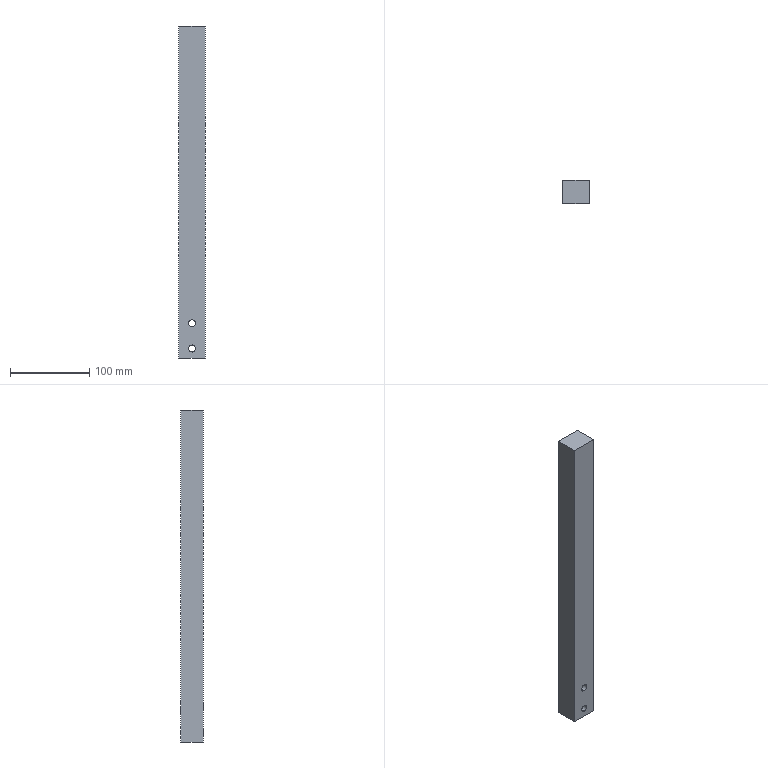Part | STEP file | zq Auxiliary Guide Rail | 1 solid | 16 faces | box 34 x 29 x 420 mm | volume 407406 mm3 | cylinder 8 | plane 8 | commonest cylinder face diameters 9 x4 16 x4
STEP:
#1=CARTESIAN_POINT('',(-17.747,48.45,16.5));
#2=VERTEX_POINT('',#1);
#3=CARTESIAN_POINT('',(-17.747,48.45,7.5));
#4=VERTEX_POINT('',#3);
#5=CARTESIAN_POINT('',(-17.747,48.45,12.));
#6=DIRECTION('',(0.,-1.,0.));
#7=DIRECTION('',(0.,0.,1.));
#8=AXIS2_PLACEMENT_3D('',#5,#6,#7);
#9=CIRCLE('',#8,4.5);
#10=EDGE_CURVE('',#2,#4,#9,.T.);
#11=ORIENTED_EDGE('',*,*,#10,.T.);
#12=CARTESIAN_POINT('',(-17.747,66.45,7.5));
#13=VERTEX_POINT('',#12);
#14=CARTESIAN_POINT('',(-17.747,47.45,7.5));
#15=DIRECTION('',(0.,1.,0.));
#16=VECTOR('',#15,1000.);
#17=LINE('',#14,#16);
#18=EDGE_CURVE('',#4,#13,#17,.T.);
#19=ORIENTED_EDGE('',*,*,#18,.T.);
#20=CARTESIAN_POINT('',(-17.747,66.45,16.5));
#21=VERTEX_POINT('',#20);
#22=CARTESIAN_POINT('',(-17.747,66.45,12.));
#23=DIRECTION('',(0.,-1.,0.));
#24=DIRECTION('',(0.,0.,1.));
#25=AXIS2_PLACEMENT_3D('',#22,#23,#24);
#26=CIRCLE('',#25,4.5);
#27=EDGE_CURVE('',#21,#13,#26,.T.);
#28=ORIENTED_EDGE('',*,*,#27,.F.);
#29=CARTESIAN_POINT('',(-17.747,47.45,16.5));
#30=DIRECTION('',(0.,1.,0.));
#31=VECTOR('',#30,1000.);
#32=LINE('',#29,#31);
#33=EDGE_CURVE('',#2,#21,#32,.T.);
#34=ORIENTED_EDGE('',*,*,#33,.F.);
#35=EDGE_LOOP('',(#11,#19,#28,#34));
#36=FACE_OUTER_BOUND('',#35,.T.);
#37=CARTESIAN_POINT('',(-17.747,47.45,12.));
#38=DIRECTION('',(0.,1.,0.));
#39=DIRECTION('',(0.,0.,1.));
#40=AXIS2_PLACEMENT_3D('',#37,#38,#39);
#41=CYLINDRICAL_SURFACE('',#40,4.5);
#42=ADVANCED_FACE('',(#36),#41,.F.);
#43=CARTESIAN_POINT('',(-17.747,48.45,48.5));
#44=VERTEX_POINT('',#43);
#45=CARTESIAN_POINT('',(-17.747,48.45,39.5));
#46=VERTEX_POINT('',#45);
#47=CARTESIAN_POINT('',(-17.747,48.45,44.));
#48=DIRECTION('',(0.,-1.,0.));
#49=DIRECTION('',(0.,0.,1.));
#50=AXIS2_PLACEMENT_3D('',#47,#48,#49);
#51=CIRCLE('',#50,4.5);
#52=EDGE_CURVE('',#44,#46,#51,.T.);
#53=ORIENTED_EDGE('',*,*,#52,.T.);
#54=CARTESIAN_POINT('',(-17.747,66.45,39.5));
#55=VERTEX_POINT('',#54);
#56=CARTESIAN_POINT('',(-17.747,47.45,39.5));
#57=DIRECTION('',(0.,1.,0.));
#58=VECTOR('',#57,1000.);
#59=LINE('',#56,#58);
#60=EDGE_CURVE('',#46,#55,#59,.T.);
#61=ORIENTED_EDGE('',*,*,#60,.T.);
#62=CARTESIAN_POINT('',(-17.747,66.45,48.5));
#63=VERTEX_POINT('',#62);
#64=CARTESIAN_POINT('',(-17.747,66.45,44.));
#65=DIRECTION('',(0.,-1.,0.));
#66=DIRECTION('',(0.,0.,1.));
#67=AXIS2_PLACEMENT_3D('',#64,#65,#66);
#68=CIRCLE('',#67,4.5);
#69=EDGE_CURVE('',#63,#55,#68,.T.);
#70=ORIENTED_EDGE('',*,*,#69,.F.);
#71=CARTESIAN_POINT('',(-17.747,47.45,48.5));
#72=DIRECTION('',(0.,1.,0.));
#73=VECTOR('',#72,1000.);
#74=LINE('',#71,#73);
#75=EDGE_CURVE('',#44,#63,#74,.T.);
#76=ORIENTED_EDGE('',*,*,#75,.F.);
#77=EDGE_LOOP('',(#53,#61,#70,#76));
#78=FACE_OUTER_BOUND('',#77,.T.);
#79=CARTESIAN_POINT('',(-17.747,47.45,44.));
#80=DIRECTION('',(0.,1.,0.));
#81=DIRECTION('',(0.,0.,1.));
#82=AXIS2_PLACEMENT_3D('',#79,#80,#81);
#83=CYLINDRICAL_SURFACE('',#82,4.5);
#84=ADVANCED_FACE('',(#78),#83,.F.);
#85=CARTESIAN_POINT('',(-17.747,66.45,36.));
#86=VERTEX_POINT('',#85);
#87=CARTESIAN_POINT('',(-17.747,66.45,52.));
#88=VERTEX_POINT('',#87);
#89=CARTESIAN_POINT('',(-17.747,66.45,44.));
#90=DIRECTION('',(0.,1.,0.));
#91=DIRECTION('',(0.,0.,1.));
#92=AXIS2_PLACEMENT_3D('',#89,#90,#91);
#93=CIRCLE('',#92,8.);
#94=EDGE_CURVE('',#86,#88,#93,.T.);
#95=ORIENTED_EDGE('',*,*,#94,.F.);
#96=CARTESIAN_POINT('',(-17.747,77.45,36.));
#97=VERTEX_POINT('',#96);
#98=CARTESIAN_POINT('',(-17.747,66.45,36.));
#99=DIRECTION('',(0.,1.,0.));
#100=VECTOR('',#99,1000.);
#101=LINE('',#98,#100);
#102=EDGE_CURVE('',#86,#97,#101,.T.);
#103=ORIENTED_EDGE('',*,*,#102,.T.);
#104=CARTESIAN_POINT('',(-17.747,77.45,52.));
#105=VERTEX_POINT('',#104);
#106=CARTESIAN_POINT('',(-17.747,77.45,44.));
#107=DIRECTION('',(0.,1.,0.));
#108=DIRECTION('',(0.,0.,1.));
#109=AXIS2_PLACEMENT_3D('',#106,#107,#108);
#110=CIRCLE('',#109,8.);
#111=EDGE_CURVE('',#97,#105,#110,.T.);
#112=ORIENTED_EDGE('',*,*,#111,.T.);
#113=CARTESIAN_POINT('',(-17.747,66.45,52.));
#114=DIRECTION('',(0.,1.,0.));
#115=VECTOR('',#114,1000.);
#116=LINE('',#113,#115);
#117=EDGE_CURVE('',#88,#105,#116,.T.);
#118=ORIENTED_EDGE('',*,*,#117,.F.);
#119=EDGE_LOOP('',(#95,#103,#112,#118));
#120=FACE_OUTER_BOUND('',#119,.T.);
#121=CARTESIAN_POINT('',(-17.747,66.45,44.));
#122=DIRECTION('',(0.,1.,0.));
#123=DIRECTION('',(0.,0.,1.));
#124=AXIS2_PLACEMENT_3D('',#121,#122,#123);
#125=CYLINDRICAL_SURFACE('',#124,8.);
#126=ADVANCED_FACE('',(#120),#125,.F.);
#127=CARTESIAN_POINT('',(-17.747,66.45,4.));
#128=VERTEX_POINT('',#127);
#129=CARTESIAN_POINT('',(-17.747,66.45,20.));
#130=VERTEX_POINT('',#129);
#131=CARTESIAN_POINT('',(-17.747,66.45,12.));
#132=DIRECTION('',(0.,1.,0.));
#133=DIRECTION('',(0.,0.,1.));
#134=AXIS2_PLACEMENT_3D('',#131,#132,#133);
#135=CIRCLE('',#134,8.);
#136=EDGE_CURVE('',#128,#130,#135,.T.);
#137=ORIENTED_EDGE('',*,*,#136,.F.);
#138=CARTESIAN_POINT('',(-17.747,77.45,4.));
#139=VERTEX_POINT('',#138);
#140=CARTESIAN_POINT('',(-17.747,66.45,4.));
#141=DIRECTION('',(0.,1.,0.));
#142=VECTOR('',#141,1000.);
#143=LINE('',#140,#142);
#144=EDGE_CURVE('',#128,#139,#143,.T.);
#145=ORIENTED_EDGE('',*,*,#144,.T.);
#146=CARTESIAN_POINT('',(-17.747,77.45,20.));
#147=VERTEX_POINT('',#146);
#148=CARTESIAN_POINT('',(-17.747,77.45,12.));
#149=DIRECTION('',(0.,1.,0.));
#150=DIRECTION('',(0.,0.,1.));
#151=AXIS2_PLACEMENT_3D('',#148,#149,#150);
#152=CIRCLE('',#151,8.);
#153=EDGE_CURVE('',#139,#147,#152,.T.);
#154=ORIENTED_EDGE('',*,*,#153,.T.);
#155=CARTESIAN_POINT('',(-17.747,66.45,20.));
#156=DIRECTION('',(0.,1.,0.));
#157=VECTOR('',#156,1000.);
#158=LINE('',#155,#157);
#159=EDGE_CURVE('',#130,#147,#158,.T.);
#160=ORIENTED_EDGE('',*,*,#159,.F.);
#161=EDGE_LOOP('',(#137,#145,#154,#160));
#162=FACE_OUTER_BOUND('',#161,.T.);
#163=CARTESIAN_POINT('',(-17.747,66.45,12.));
#164=DIRECTION('',(0.,1.,0.));
#165=DIRECTION('',(0.,0.,1.));
#166=AXIS2_PLACEMENT_3D('',#163,#164,#165);
#167=CYLINDRICAL_SURFACE('',#166,8.);
#168=ADVANCED_FACE('',(#162),#167,.F.);
#169=CARTESIAN_POINT('',(-0.7466,48.45,420.));
#170=VERTEX_POINT('',#169);
#171=CARTESIAN_POINT('',(-0.7466,48.45,0.));
#172=VERTEX_POINT('',#171);
#173=CARTESIAN_POINT('',(-0.7466,48.45,420.));
#174=DIRECTION('',(0.,0.,-1.));
#175=VECTOR('',#174,1000.);
#176=LINE('',#173,#175);
#177=EDGE_CURVE('',#170,#172,#176,.T.);
#178=ORIENTED_EDGE('',*,*,#177,.F.);
#179=CARTESIAN_POINT('',(-34.747,48.45,420.));
#180=VERTEX_POINT('',#179);
#181=CARTESIAN_POINT('',(-34.747,48.45,420.));
#182=DIRECTION('',(1.,0.,0.));
#183=VECTOR('',#182,1000.);
#184=LINE('',#181,#183);
#185=EDGE_CURVE('',#180,#170,#184,.T.);
#186=ORIENTED_EDGE('',*,*,#185,.F.);
#187=CARTESIAN_POINT('',(-34.747,48.45,0.));
#188=VERTEX_POINT('',#187);
#189=CARTESIAN_POINT('',(-34.747,48.45,420.));
#190=DIRECTION('',(0.,0.,1.));
#191=VECTOR('',#190,1000.);
#192=LINE('',#189,#191);
#193=EDGE_CURVE('',#188,#180,#192,.T.);
#194=ORIENTED_EDGE('',*,*,#193,.F.);
#195=CARTESIAN_POINT('',(-34.747,48.45,0.));
#196=DIRECTION('',(-1.,0.,0.));
#197=VECTOR('',#196,1000.);
#198=LINE('',#195,#197);
#199=EDGE_CURVE('',#172,#188,#198,.T.);
#200=ORIENTED_EDGE('',*,*,#199,.F.);
#201=EDGE_LOOP('',(#178,#186,#194,#200));
#202=FACE_OUTER_BOUND('',#201,.T.);
#203=ORIENTED_EDGE('',*,*,#10,.F.);
#204=CARTESIAN_POINT('',(-17.747,48.45,12.));
#205=DIRECTION('',(0.,-1.,0.));
#206=DIRECTION('',(0.,0.,1.));
#207=AXIS2_PLACEMENT_3D('',#204,#205,#206);
#208=CIRCLE('',#207,4.5);
#209=EDGE_CURVE('',#4,#2,#208,.T.);
#210=ORIENTED_EDGE('',*,*,#209,.F.);
#211=EDGE_LOOP('',(#203,#210));
#212=FACE_BOUND('',#211,.T.);
#213=ORIENTED_EDGE('',*,*,#52,.F.);
#214=CARTESIAN_POINT('',(-17.747,48.45,44.));
#215=DIRECTION('',(0.,-1.,0.));
#216=DIRECTION('',(0.,0.,1.));
#217=AXIS2_PLACEMENT_3D('',#214,#215,#216);
#218=CIRCLE('',#217,4.5);
#219=EDGE_CURVE('',#46,#44,#218,.T.);
#220=ORIENTED_EDGE('',*,*,#219,.F.);
#221=EDGE_LOOP('',(#213,#220));
#222=FACE_BOUND('',#221,.T.);
#223=CARTESIAN_POINT('',(-34.747,48.45,420.));
#224=DIRECTION('',(0.,1.,0.));
#225=DIRECTION('',(0.,0.,1.));
#226=AXIS2_PLACEMENT_3D('',#223,#224,#225);
#227=PLANE('',#226);
#228=ADVANCED_FACE('',(#202,#212,#222),#227,.F.);
#229=CARTESIAN_POINT('',(-0.7466,77.45,0.));
#230=VERTEX_POINT('',#229);
#231=CARTESIAN_POINT('',(-34.747,77.45,0.));
#232=VERTEX_POINT('',#231);
#233=CARTESIAN_POINT('',(0.,77.45,0.));
#234=DIRECTION('',(-1.,0.,0.));
#235=VECTOR('',#234,1000.);
#236=LINE('',#233,#235);
#237=EDGE_CURVE('',#230,#232,#236,.T.);
#238=ORIENTED_EDGE('',*,*,#237,.F.);
#239=CARTESIAN_POINT('',(-0.7466,0.,0.));
#240=DIRECTION('',(0.,1.,0.));
#241=VECTOR('',#240,1000.);
#242=LINE('',#239,#241);
#243=EDGE_CURVE('',#172,#230,#242,.T.);
#244=ORIENTED_EDGE('',*,*,#243,.F.);
#245=ORIENTED_EDGE('',*,*,#199,.T.);
#246=CARTESIAN_POINT('',(-34.747,0.,0.));
#247=DIRECTION('',(0.,-1.,0.));
#248=VECTOR('',#247,1000.);
#249=LINE('',#246,#248);
#250=EDGE_CURVE('',#232,#188,#249,.T.);
#251=ORIENTED_EDGE('',*,*,#250,.F.);
#252=EDGE_LOOP('',(#238,#244,#245,#251));
#253=FACE_OUTER_BOUND('',#252,.T.);
#254=CARTESIAN_POINT('',(0.,0.,0.));
#255=DIRECTION('',(0.,0.,1.));
#256=DIRECTION('',(1.,0.,0.));
#257=AXIS2_PLACEMENT_3D('',#254,#255,#256);
#258=PLANE('',#257);
#259=ADVANCED_FACE('',(#253),#258,.F.);
#260=CARTESIAN_POINT('',(-0.7466,77.45,420.));
#261=VERTEX_POINT('',#260);
#262=CARTESIAN_POINT('',(-0.7466,77.45,420.));
#263=DIRECTION('',(0.,0.,-1.));
#264=VECTOR('',#263,1000.);
#265=LINE('',#262,#264);
#266=EDGE_CURVE('',#261,#230,#265,.T.);
#267=ORIENTED_EDGE('',*,*,#266,.F.);
#268=CARTESIAN_POINT('',(-0.7466,77.45,420.));
#269=DIRECTION('',(0.,1.,0.));
#270=VECTOR('',#269,1000.);
#271=LINE('',#268,#270);
#272=EDGE_CURVE('',#170,#261,#271,.T.);
#273=ORIENTED_EDGE('',*,*,#272,.F.);
#274=ORIENTED_EDGE('',*,*,#177,.T.);
#275=ORIENTED_EDGE('',*,*,#243,.T.);
#276=EDGE_LOOP('',(#267,#273,#274,#275));
#277=FACE_OUTER_BOUND('',#276,.T.);
#278=CARTESIAN_POINT('',(-0.7466,77.45,420.));
#279=DIRECTION('',(-1.,0.,0.));
#280=DIRECTION('',(0.,-1.,0.));
#281=AXIS2_PLACEMENT_3D('',#278,#279,#280);
#282=PLANE('',#281);
#283=ADVANCED_FACE('',(#277),#282,.F.);
#284=ORIENTED_EDGE('',*,*,#272,.T.);
#285=CARTESIAN_POINT('',(-34.747,77.45,420.));
#286=VERTEX_POINT('',#285);
#287=CARTESIAN_POINT('',(0.,77.45,420.));
#288=DIRECTION('',(-1.,0.,0.));
#289=VECTOR('',#288,1000.);
#290=LINE('',#287,#289);
#291=EDGE_CURVE('',#261,#286,#290,.T.);
#292=ORIENTED_EDGE('',*,*,#291,.T.);
#293=CARTESIAN_POINT('',(-34.747,0.,420.));
#294=DIRECTION('',(0.,-1.,0.));
#295=VECTOR('',#294,1000.);
#296=LINE('',#293,#295);
#297=EDGE_CURVE('',#286,#180,#296,.T.);
#298=ORIENTED_EDGE('',*,*,#297,.T.);
#299=ORIENTED_EDGE('',*,*,#185,.T.);
#300=EDGE_LOOP('',(#284,#292,#298,#299));
#301=FACE_OUTER_BOUND('',#300,.T.);
#302=CARTESIAN_POINT('',(0.,0.,420.));
#303=DIRECTION('',(0.,0.,1.));
#304=DIRECTION('',(1.,0.,0.));
#305=AXIS2_PLACEMENT_3D('',#302,#303,#304);
#306=PLANE('',#305);
#307=ADVANCED_FACE('',(#301),#306,.T.);
#308=ORIENTED_EDGE('',*,*,#193,.T.);
#309=ORIENTED_EDGE('',*,*,#297,.F.);
#310=CARTESIAN_POINT('',(-34.747,77.45,420.));
#311=DIRECTION('',(0.,0.,1.));
#312=VECTOR('',#311,1000.);
#313=LINE('',#310,#312);
#314=EDGE_CURVE('',#232,#286,#313,.T.);
#315=ORIENTED_EDGE('',*,*,#314,.F.);
#316=ORIENTED_EDGE('',*,*,#250,.T.);
#317=EDGE_LOOP('',(#308,#309,#315,#316));
#318=FACE_OUTER_BOUND('',#317,.T.);
#319=CARTESIAN_POINT('',(-34.747,77.45,420.));
#320=DIRECTION('',(1.,0.,0.));
#321=DIRECTION('',(0.,1.,0.));
#322=AXIS2_PLACEMENT_3D('',#319,#320,#321);
#323=PLANE('',#322);
#324=ADVANCED_FACE('',(#318),#323,.F.);
#325=ORIENTED_EDGE('',*,*,#18,.F.);
#326=ORIENTED_EDGE('',*,*,#209,.T.);
#327=ORIENTED_EDGE('',*,*,#33,.T.);
#328=CARTESIAN_POINT('',(-17.747,66.45,12.));
#329=DIRECTION('',(0.,-1.,0.));
#330=DIRECTION('',(0.,0.,1.));
#331=AXIS2_PLACEMENT_3D('',#328,#329,#330);
#332=CIRCLE('',#331,4.5);
#333=EDGE_CURVE('',#13,#21,#332,.T.);
#334=ORIENTED_EDGE('',*,*,#333,.F.);
#335=EDGE_LOOP('',(#325,#326,#327,#334));
#336=FACE_OUTER_BOUND('',#335,.T.);
#337=CARTESIAN_POINT('',(-17.747,47.45,12.));
#338=DIRECTION('',(0.,1.,0.));
#339=DIRECTION('',(0.,0.,1.));
#340=AXIS2_PLACEMENT_3D('',#337,#338,#339);
#341=CYLINDRICAL_SURFACE('',#340,4.5);
#342=ADVANCED_FACE('',(#336),#341,.F.);
#343=ORIENTED_EDGE('',*,*,#60,.F.);
#344=ORIENTED_EDGE('',*,*,#219,.T.);
#345=ORIENTED_EDGE('',*,*,#75,.T.);
#346=CARTESIAN_POINT('',(-17.747,66.45,44.));
#347=DIRECTION('',(0.,-1.,0.));
#348=DIRECTION('',(0.,0.,1.));
#349=AXIS2_PLACEMENT_3D('',#346,#347,#348);
#350=CIRCLE('',#349,4.5);
#351=EDGE_CURVE('',#55,#63,#350,.T.);
#352=ORIENTED_EDGE('',*,*,#351,.F.);
#353=EDGE_LOOP('',(#343,#344,#345,#352));
#354=FACE_OUTER_BOUND('',#353,.T.);
#355=CARTESIAN_POINT('',(-17.747,47.45,44.));
#356=DIRECTION('',(0.,1.,0.));
#357=DIRECTION('',(0.,0.,1.));
#358=AXIS2_PLACEMENT_3D('',#355,#356,#357);
#359=CYLINDRICAL_SURFACE('',#358,4.5);
#360=ADVANCED_FACE('',(#354),#359,.F.);
#361=ORIENTED_EDGE('',*,*,#314,.T.);
#362=ORIENTED_EDGE('',*,*,#291,.F.);
#363=ORIENTED_EDGE('',*,*,#266,.T.);
#364=ORIENTED_EDGE('',*,*,#237,.T.);
#365=EDGE_LOOP('',(#361,#362,#363,#364));
#366=FACE_OUTER_BOUND('',#365,.T.);
#367=CARTESIAN_POINT('',(-17.747,77.45,44.));
#368=DIRECTION('',(0.,1.,0.));
#369=DIRECTION('',(0.,0.,1.));
#370=AXIS2_PLACEMENT_3D('',#367,#368,#369);
#371=CIRCLE('',#370,8.);
#372=EDGE_CURVE('',#105,#97,#371,.T.);
#373=ORIENTED_EDGE('',*,*,#372,.F.);
#374=ORIENTED_EDGE('',*,*,#111,.F.);
#375=EDGE_LOOP('',(#373,#374));
#376=FACE_BOUND('',#375,.T.);
#377=CARTESIAN_POINT('',(-17.747,77.45,12.));
#378=DIRECTION('',(0.,1.,0.));
#379=DIRECTION('',(0.,0.,1.));
#380=AXIS2_PLACEMENT_3D('',#377,#378,#379);
#381=CIRCLE('',#380,8.);
#382=EDGE_CURVE('',#147,#139,#381,.T.);
#383=ORIENTED_EDGE('',*,*,#382,.F.);
#384=ORIENTED_EDGE('',*,*,#153,.F.);
#385=EDGE_LOOP('',(#383,#384));
#386=FACE_BOUND('',#385,.T.);
#387=CARTESIAN_POINT('',(-34.747,77.45,420.));
#388=DIRECTION('',(0.,-1.,0.));
#389=DIRECTION('',(0.,0.,-1.));
#390=AXIS2_PLACEMENT_3D('',#387,#388,#389);
#391=PLANE('',#390);
#392=ADVANCED_FACE('',(#366,#376,#386),#391,.F.);
#393=ORIENTED_EDGE('',*,*,#27,.T.);
#394=ORIENTED_EDGE('',*,*,#333,.T.);
#395=EDGE_LOOP('',(#393,#394));
#396=FACE_BOUND('',#395,.T.);
#397=CARTESIAN_POINT('',(-17.747,66.45,12.));
#398=DIRECTION('',(0.,1.,0.));
#399=DIRECTION('',(0.,0.,1.));
#400=AXIS2_PLACEMENT_3D('',#397,#398,#399);
#401=CIRCLE('',#400,8.);
#402=EDGE_CURVE('',#130,#128,#401,.T.);
#403=ORIENTED_EDGE('',*,*,#402,.T.);
#404=ORIENTED_EDGE('',*,*,#136,.T.);
#405=EDGE_LOOP('',(#403,#404));
#406=FACE_OUTER_BOUND('',#405,.T.);
#407=CARTESIAN_POINT('',(-17.747,66.45,12.));
#408=DIRECTION('',(0.,1.,0.));
#409=DIRECTION('',(0.,0.,1.));
#410=AXIS2_PLACEMENT_3D('',#407,#408,#409);
#411=PLANE('',#410);
#412=ADVANCED_FACE('',(#396,#406),#411,.T.);
#413=ORIENTED_EDGE('',*,*,#69,.T.);
#414=ORIENTED_EDGE('',*,*,#351,.T.);
#415=EDGE_LOOP('',(#413,#414));
#416=FACE_BOUND('',#415,.T.);
#417=CARTESIAN_POINT('',(-17.747,66.45,44.));
#418=DIRECTION('',(0.,1.,0.));
#419=DIRECTION('',(0.,0.,1.));
#420=AXIS2_PLACEMENT_3D('',#417,#418,#419);
#421=CIRCLE('',#420,8.);
#422=EDGE_CURVE('',#88,#86,#421,.T.);
#423=ORIENTED_EDGE('',*,*,#422,.T.);
#424=ORIENTED_EDGE('',*,*,#94,.T.);
#425=EDGE_LOOP('',(#423,#424));
#426=FACE_OUTER_BOUND('',#425,.T.);
#427=CARTESIAN_POINT('',(-17.747,66.45,44.));
#428=DIRECTION('',(0.,1.,0.));
#429=DIRECTION('',(0.,0.,1.));
#430=AXIS2_PLACEMENT_3D('',#427,#428,#429);
#431=PLANE('',#430);
#432=ADVANCED_FACE('',(#416,#426),#431,.T.);
#433=ORIENTED_EDGE('',*,*,#102,.F.);
#434=ORIENTED_EDGE('',*,*,#422,.F.);
#435=ORIENTED_EDGE('',*,*,#117,.T.);
#436=ORIENTED_EDGE('',*,*,#372,.T.);
#437=EDGE_LOOP('',(#433,#434,#435,#436));
#438=FACE_OUTER_BOUND('',#437,.T.);
#439=CARTESIAN_POINT('',(-17.747,66.45,44.));
#440=DIRECTION('',(0.,1.,0.));
#441=DIRECTION('',(0.,0.,1.));
#442=AXIS2_PLACEMENT_3D('',#439,#440,#441);
#443=CYLINDRICAL_SURFACE('',#442,8.);
#444=ADVANCED_FACE('',(#438),#443,.F.);
#445=ORIENTED_EDGE('',*,*,#144,.F.);
#446=ORIENTED_EDGE('',*,*,#402,.F.);
#447=ORIENTED_EDGE('',*,*,#159,.T.);
#448=ORIENTED_EDGE('',*,*,#382,.T.);
#449=EDGE_LOOP('',(#445,#446,#447,#448));
#450=FACE_OUTER_BOUND('',#449,.T.);
#451=CARTESIAN_POINT('',(-17.747,66.45,12.));
#452=DIRECTION('',(0.,1.,0.));
#453=DIRECTION('',(0.,0.,1.));
#454=AXIS2_PLACEMENT_3D('',#451,#452,#453);
#455=CYLINDRICAL_SURFACE('',#454,8.);
#456=ADVANCED_FACE('',(#450),#455,.F.);
#457=CLOSED_SHELL('',(#42,#84,#126,#168,#228,#259,#283,#307,#324,#342,#360,#392,#412,#432,#444,#456));
#458=MANIFOLD_SOLID_BREP('',#457);
#459=CARTESIAN_POINT('',(0.,0.,0.));
#460=DIRECTION('',(0.,0.,1.));
#461=DIRECTION('',(1.,0.,0.));
#462=AXIS2_PLACEMENT_3D('',#459,#460,#461);
#463=(LENGTH_UNIT()NAMED_UNIT(*)SI_UNIT(.MILLI.,.METRE.));
#464=UNCERTAINTY_MEASURE_WITH_UNIT(LENGTH_MEASURE(0.00001),#463,'','');
#465=(NAMED_UNIT(*)PLANE_ANGLE_UNIT()SI_UNIT($,.RADIAN.));
#466=(NAMED_UNIT(*)SI_UNIT($,.STERADIAN.)SOLID_ANGLE_UNIT());
#467=(GEOMETRIC_REPRESENTATION_CONTEXT(3)GLOBAL_UNCERTAINTY_ASSIGNED_CONTEXT((#464))GLOBAL_UNIT_ASSIGNED_CONTEXT((#463,#465,#466))REPRESENTATION_CONTEXT('',''));
#468=ADVANCED_BREP_SHAPE_REPRESENTATION('',(#458,#462),#467);